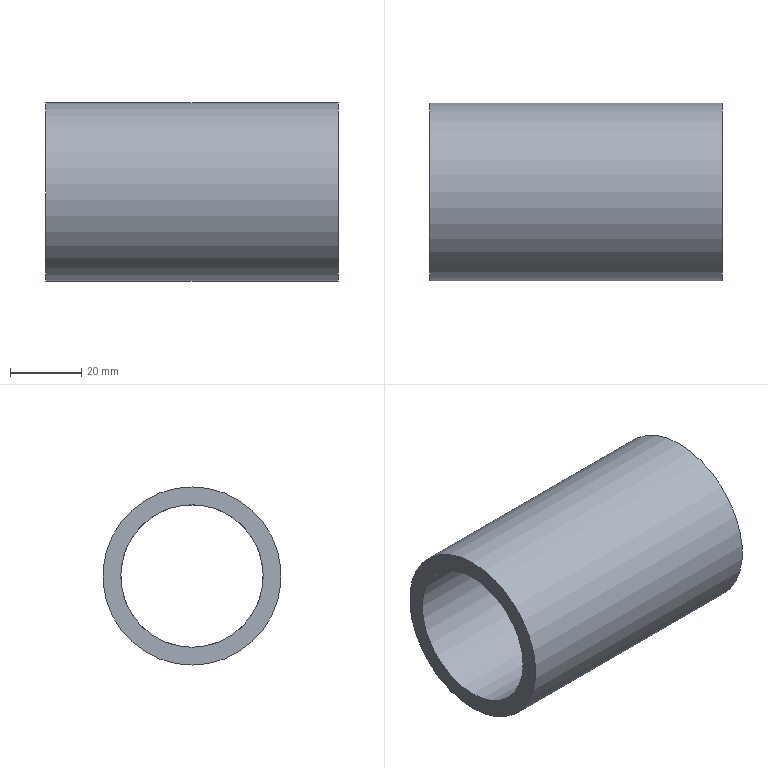Part | STEP file | solid 50 | 1 solid | 4 faces | box 82 x 50 x 50 mm | volume 57962 mm3 | plane 2 | cylinder 2 | commonest cylinder face diameters 40 x1 50 x1